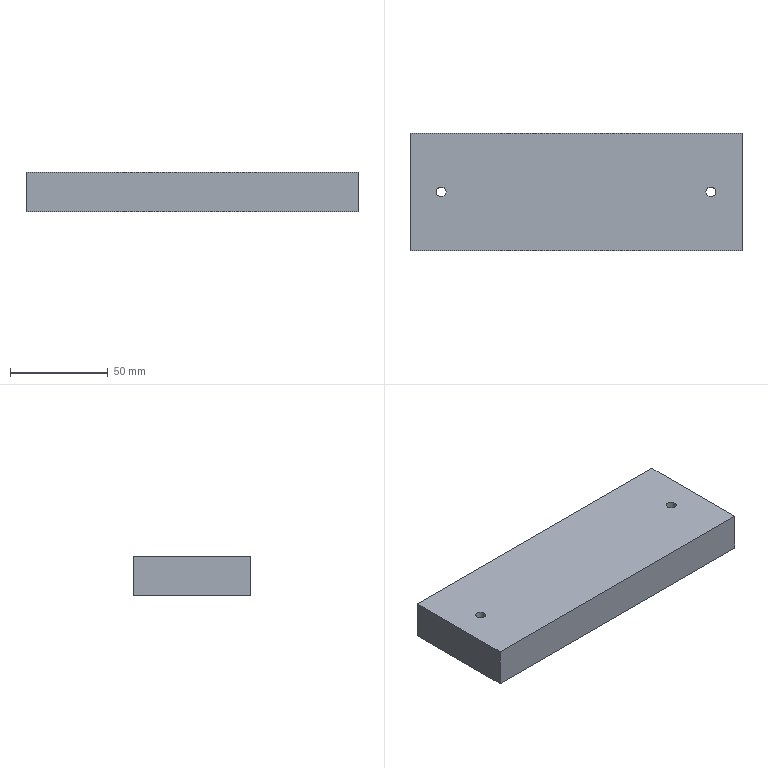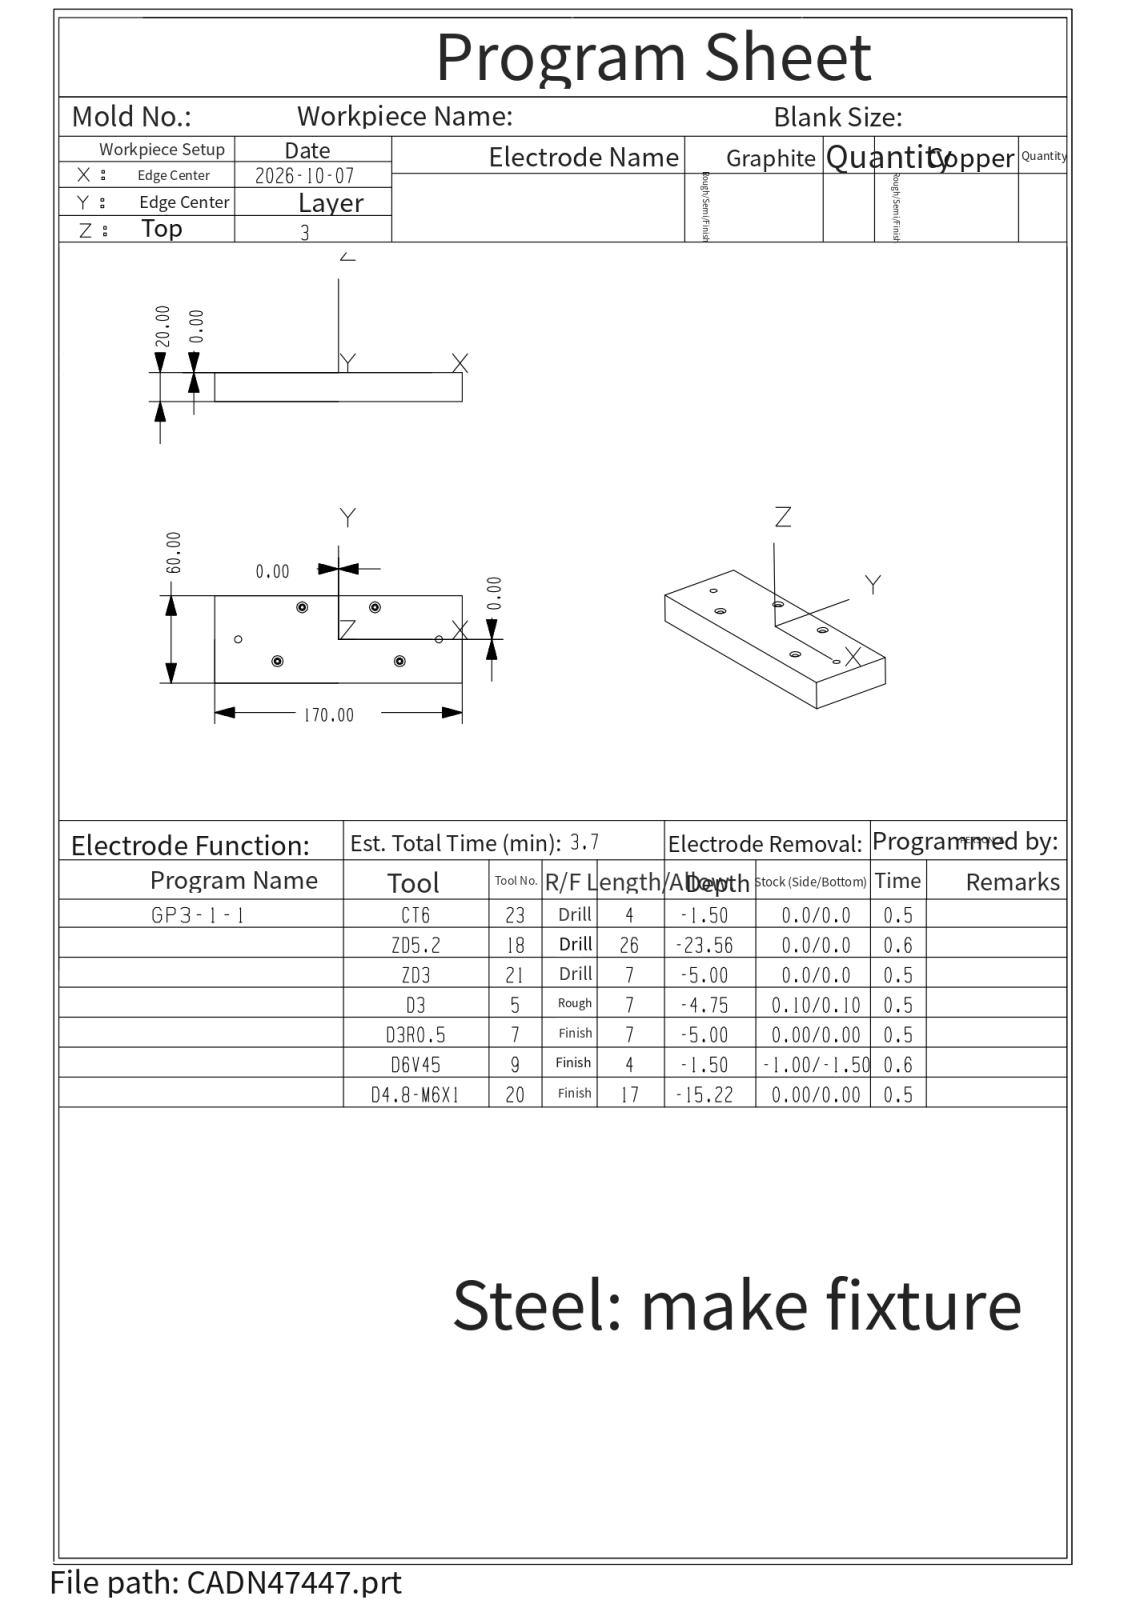NC program | NX | posted by the shop | part box 170 x 60 x 20 mm
Lines 3043 to 4032 of 14163:
T07 M06
T09
( name=D3R0.5    T=7 )
( XY = 0.00 )
( Z = 0.00 )
G00 G90 G54 X-42.899 Y-16.408 S8000 M03
G43 Z10. H07 M08
Z.186
G01 Z-.014 F2400.
Y-16.671
G03 X-41.999 Y-17.571 I.9 J0.0
I0.0 J2.571 F3000.
G01 X-41.917 Y-17.564
X-41.835 Y-17.554 Z-.015
X-41.754 Y-17.542 Z-.016
X-41.673 Y-17.527
X-41.593 Y-17.51 Z-.017
X-41.514 Y-17.49 Z-.018
X-41.436 Y-17.468 Z-.019
X-41.358 Y-17.444
X-41.282 Y-17.417 Z-.02
X-41.206 Y-17.388 Z-.021
X-41.131 Y-17.357
X-41.058 Y-17.323 Z-.022
X-40.986 Y-17.288 Z-.023
X-40.915 Y-17.25 Z-.024
X-40.846 Y-17.21
X-40.778 Y-17.168 Z-.025
X-40.711 Y-17.124 Z-.026
X-40.646 Y-17.077 Z-.027
X-40.583 Y-17.029
X-40.521 Y-16.98 Z-.028
X-40.461 Y-16.928 Z-.029
X-40.402 Y-16.874
X-40.346 Y-16.819 Z-.03
X-40.291 Y-16.762 Z-.031
X-40.239 Y-16.704 Z-.032
X-40.188 Y-16.644
X-40.139 Y-16.582 Z-.033
X-40.092 Y-16.519 Z-.034
X-40.048 Y-16.455
X-40.005 Y-16.389 Z-.035
X-39.965 Y-16.323 Z-.036
X-39.926 Y-16.255 Z-.037
X-39.89 Y-16.186
X-39.857 Y-16.116 Z-.038
G03 X-41.999 Y-17.416 I-2.142 J1.116
G01 X-41.915 Y-17.411 Z-.039
X-41.83 Y-17.402 Z-.04
X-41.747 Y-17.391
X-41.663 Y-17.377 Z-.041
X-41.581 Y-17.361 Z-.042
X-41.499 Y-17.341
X-41.418 Y-17.319 Z-.043
X-41.338 Y-17.294 Z-.044
X-41.259 Y-17.266 Z-.045
X-41.181 Y-17.235
X-41.105 Y-17.202 Z-.046
X-41.029 Y-17.166 Z-.047
X-40.955 Y-17.128 Z-.048
X-40.883 Y-17.087
X-40.812 Y-17.044 Z-.049
X-40.743 Y-16.998 Z-.05
X-40.675 Y-16.95 Z-.051
X-40.61 Y-16.9
X-40.546 Y-16.847 Z-.052
X-40.484 Y-16.793 Z-.053
X-40.424 Y-16.736 Z-.054
X-40.366 Y-16.678
X-40.311 Y-16.617 Z-.055
X-40.257 Y-16.555 Z-.056
X-40.206 Y-16.491 Z-.057
X-40.157 Y-16.425
X-40.111 Y-16.358 Z-.058
X-40.067 Y-16.289 Z-.059
X-40.026 Y-16.219
X-39.987 Y-16.148 Z-.06
X-39.95 Y-16.075 Z-.061
X-39.916 Y-16.001 Z-.062
X-39.885 Y-15.926
X-39.857 Y-15.851 Z-.063
X-39.831 Y-15.774 Z-.064
X-39.808 Y-15.697 Z-.065
X-39.787 Y-15.619
X-39.77 Y-15.54 Z-.066
X-39.755 Y-15.461 Z-.067
X-39.743 Y-15.381 Z-.068
X-39.734 Y-15.302
X-39.727 Y-15.222 Z-.069
X-39.724 Y-15.142 Z-.07
X-39.723 Y-15.062 Z-.071
X-39.725 Y-14.982
X-39.729 Y-14.902 Z-.072
X-39.737 Y-14.823 Z-.073
X-39.747 Y-14.744 Z-.074
G03 X-41.999 Y-17.267 I-2.252 J-.256
G01 X-41.914 Y-17.262
X-41.829 Y-17.255 Z-.075
X-41.744 Y-17.244 Z-.076
X-41.66 Y-17.23 Z-.077
X-41.576 Y-17.213
X-41.493 Y-17.193 Z-.078
X-41.412 Y-17.17 Z-.079
X-41.331 Y-17.144 Z-.08
X-41.251 Y-17.115
X-41.173 Y-17.083 Z-.081
X-41.096 Y-17.048 Z-.082
X-41.02 Y-17.01 Z-.083
X-40.946 Y-16.969
X-40.874 Y-16.926 Z-.084
X-40.803 Y-16.88 Z-.085
X-40.735 Y-16.831
X-40.668 Y-16.78 Z-.086
X-40.603 Y-16.727 Z-.087
X-40.541 Y-16.671 Z-.088
X-40.48 Y-16.613
X-40.422 Y-16.553 Z-.089
X-40.366 Y-16.49 Z-.09
X-40.313 Y-16.426 Z-.091
X-40.262 Y-16.36
X-40.214 Y-16.292 Z-.092
X-40.169 Y-16.222 Z-.093
X-40.126 Y-16.151 Z-.094
X-40.086 Y-16.078
X-40.048 Y-16.004 Z-.095
X-40.014 Y-15.929 Z-.096
X-39.982 Y-15.853 Z-.097
X-39.954 Y-15.775
X-39.928 Y-15.696 Z-.098
X-39.906 Y-15.617 Z-.099
X-39.886 Y-15.537 Z-.1
X-39.869 Y-15.456
X-39.856 Y-15.375 Z-.101
X-39.846 Y-15.294 Z-.102
X-39.838 Y-15.212 Z-.103
X-39.834 Y-15.13
X-39.833 Y-15.048 Z-.104
X-39.835 Y-14.966 Z-.105
X-39.84 Y-14.885 Z-.106
X-39.848 Y-14.803
X-39.859 Y-14.723 Z-.107
X-39.873 Y-14.642 Z-.108
X-39.89 Y-14.563 Z-.109
X-39.91 Y-14.484
X-39.933 Y-14.406 Z-.11
X-39.959 Y-14.329 Z-.111
X-39.988 Y-14.253 Z-.112
X-40.02 Y-14.179
X-40.054 Y-14.106 Z-.113
X-40.091 Y-14.034 Z-.114
X-40.131 Y-13.963 Z-.115
X-40.173 Y-13.895
X-40.218 Y-13.828 Z-.116
X-40.265 Y-13.762 Z-.117
X-40.315 Y-13.699 Z-.118
X-40.367 Y-13.638
X-40.421 Y-13.579 Z-.119
X-40.477 Y-13.521 Z-.12
G03 X-41.999 Y-17.122 I-1.522 J-1.479
G01 X-41.914 Y-17.118 Z-.121
X-41.828 Y-17.111
X-41.743 Y-17.1 Z-.122
X-41.659 Y-17.086 Z-.123
X-41.575 Y-17.069 Z-.124
X-41.492 Y-17.048
X-41.411 Y-17.024 Z-.125
X-41.33 Y-16.996 Z-.126
X-41.251 Y-16.966 Z-.127
X-41.172 Y-16.932
X-41.096 Y-16.895 Z-.128
X-41.021 Y-16.856 Z-.129
X-40.948 Y-16.813 Z-.13
X-40.876 Y-16.767
X-40.807 Y-16.719 Z-.131
X-40.74 Y-16.668 Z-.132
X-40.675 Y-16.614 Z-.133
X-40.612 Y-16.558
X-40.551 Y-16.499 Z-.134
X-40.493 Y-16.438 Z-.135
X-40.438 Y-16.374 Z-.136
X-40.385 Y-16.309
X-40.335 Y-16.241 Z-.137
X-40.288 Y-16.172 Z-.138
X-40.243 Y-16.101 Z-.139
X-40.202 Y-16.028
X-40.164 Y-15.954 Z-.14
X-40.128 Y-15.878 Z-.141
X-40.096 Y-15.801 Z-.142
X-40.067 Y-15.723
X-40.041 Y-15.643 Z-.143
X-40.018 Y-15.563 Z-.144
X-39.999 Y-15.482 Z-.145
X-39.983 Y-15.401
X-39.97 Y-15.319 Z-.146
X-39.961 Y-15.236 Z-.147
X-39.955 Y-15.153 Z-.148
X-39.952 Y-15.071
X-39.953 Y-14.988 Z-.149
X-39.957 Y-14.905 Z-.15
X-39.964 Y-14.823 Z-.151
X-39.975 Y-14.741
X-39.989 Y-14.66 Z-.152
X-40.006 Y-14.579 Z-.153
X-40.026 Y-14.499 Z-.154
X-40.05 Y-14.42
X-40.077 Y-14.343 Z-.155
X-40.106 Y-14.266 Z-.156
X-40.139 Y-14.191 Z-.157
X-40.175 Y-14.117
X-40.214 Y-14.045 Z-.158
X-40.255 Y-13.975 Z-.159
X-40.3 Y-13.906 Z-.16
X-40.347 Y-13.839
X-40.396 Y-13.774 Z-.161
X-40.449 Y-13.712 Z-.162
X-40.503 Y-13.651 Z-.163
X-40.56 Y-13.593
X-40.619 Y-13.537 Z-.164
X-40.681 Y-13.484 Z-.165
X-40.744 Y-13.433 Z-.166
X-40.81 Y-13.385
X-40.877 Y-13.34 Z-.167
X-40.946 Y-13.297 Z-.168
X-41.016 Y-13.258 Z-.169
X-41.088 Y-13.221
X-41.162 Y-13.187 Z-.17
X-41.236 Y-13.156 Z-.171
X-41.312 Y-13.129 Z-.172
X-41.389 Y-13.104
X-41.466 Y-13.082 Z-.173
X-41.545 Y-13.064 Z-.174
X-41.623 Y-13.049 Z-.175
X-41.703 Y-13.037
X-41.783 Y-13.028 Z-.176
X-41.863 Y-13.023 Z-.177
G03 X-41.999 Y-16.982 I-.136 J-1.977
G01 X-41.914 Y-16.978 Z-.178
X-41.829 Y-16.971
X-41.744 Y-16.96 Z-.179
X-41.66 Y-16.946 Z-.18
X-41.577 Y-16.928
X-41.495 Y-16.906 Z-.181
X-41.413 Y-16.881 Z-.182
X-41.333 Y-16.853 Z-.183
X-41.255 Y-16.821
X-41.178 Y-16.786 Z-.184
X-41.102 Y-16.747 Z-.185
X-41.028 Y-16.705 Z-.186
X-40.957 Y-16.661
X-40.887 Y-16.613 Z-.187
X-40.82 Y-16.562 Z-.188
X-40.754 Y-16.509 Z-.189
X-40.691 Y-16.452
X-40.631 Y-16.393 Z-.19
X-40.574 Y-16.332 Z-.191
X-40.519 Y-16.268 Z-.192
X-40.467 Y-16.202
X-40.417 Y-16.134 Z-.193
X-40.371 Y-16.064 Z-.194
X-40.328 Y-15.992 Z-.195
X-40.288 Y-15.919
X-40.252 Y-15.843 Z-.196
X-40.219 Y-15.767 Z-.197
X-40.189 Y-15.688 Z-.198
X-40.162 Y-15.609
X-40.139 Y-15.529 Z-.199
X-40.119 Y-15.448 Z-.2
X-40.103 Y-15.366 Z-.201
X-40.091 Y-15.284
X-40.082 Y-15.201 Z-.202
X-40.077 Y-15.118 Z-.203
X-40.075 Y-15.035 Z-.204
X-40.077 Y-14.952
X-40.082 Y-14.87 Z-.205
X-40.091 Y-14.787 Z-.206
X-40.103 Y-14.705 Z-.207
X-40.119 Y-14.624
X-40.139 Y-14.544 Z-.208
X-40.161 Y-14.465 Z-.209
X-40.188 Y-14.386 Z-.21
X-40.217 Y-14.309
X-40.25 Y-14.234 Z-.211
X-40.286 Y-14.16 Z-.212
X-40.325 Y-14.087 Z-.213
X-40.367 Y-14.017
X-40.412 Y-13.948 Z-.214
X-40.46 Y-13.882 Z-.215
X-40.511 Y-13.817 Z-.216
X-40.565 Y-13.755
X-40.621 Y-13.696 Z-.217
X-40.679 Y-13.638 Z-.218
X-40.74 Y-13.584 Z-.219
X-40.803 Y-13.532
X-40.869 Y-13.483 Z-.22
X-40.936 Y-13.437 Z-.221
X-41.005 Y-13.394 Z-.222
X-41.076 Y-13.354
X-41.148 Y-13.317 Z-.223
X-41.222 Y-13.283 Z-.224
X-41.298 Y-13.252
X-41.374 Y-13.225 Z-.225
X-41.452 Y-13.201 Z-.226
X-41.53 Y-13.181 Z-.227
X-41.609 Y-13.163
X-41.689 Y-13.15 Z-.228
X-41.769 Y-13.139 Z-.229
X-41.85 Y-13.133 Z-.23
X-41.93 Y-13.129
X-42.011 Y-13.13 Z-.231
X-42.092 Y-13.133 Z-.232
X-42.172 Y-13.14 Z-.233
X-42.252 Y-13.151
X-42.331 Y-13.165 Z-.234
X-42.409 Y-13.182 Z-.235
X-42.487 Y-13.203 Z-.236
X-42.564 Y-13.227
X-42.639 Y-13.254 Z-.237
X-42.713 Y-13.285 Z-.238
X-42.786 Y-13.318 Z-.239
X-42.857 Y-13.355
X-42.926 Y-13.395 Z-.24
X-42.994 Y-13.438 Z-.241
X-43.06 Y-13.483 Z-.242
X-43.123 Y-13.531
X-43.185 Y-13.582 Z-.243
X-43.244 Y-13.636 Z-.244
G03 X-41.999 Y-16.847 I1.245 J-1.364
G01 X-41.913 Y-16.843 Z-.245
X-41.828 Y-16.836 Z-.246
X-41.742 Y-16.824
X-41.658 Y-16.809 Z-.247
X-41.574 Y-16.79 Z-.248
X-41.492 Y-16.766 Z-.249
X-41.411 Y-16.739 Z-.25
X-41.331 Y-16.709
X-41.252 Y-16.674 Z-.251
X-41.176 Y-16.636 Z-.252
X-41.101 Y-16.595 Z-.253
X-41.029 Y-16.55 Z-.254
X-40.958 Y-16.502 Z-.255
X-40.89 Y-16.451
X-40.825 Y-16.396 Z-.256
X-40.762 Y-16.339 Z-.257
X-40.702 Y-16.279 Z-.258
X-40.645 Y-16.216 Z-.259
X-40.591 Y-16.151
X-40.54 Y-16.083 Z-.26
X-40.492 Y-16.013 Z-.261
X-40.448 Y-15.941 Z-.262
X-40.407 Y-15.867 Z-.263
X-40.369 Y-15.791 Z-.264
X-40.336 Y-15.714
X-40.306 Y-15.635 Z-.265
X-40.279 Y-15.555 Z-.266
X-40.257 Y-15.474 Z-.267
X-40.238 Y-15.392 Z-.268
X-40.223 Y-15.309
X-40.212 Y-15.226 Z-.269
X-40.205 Y-15.142 Z-.27
X-40.201 Y-15.058 Z-.271
X-40.202 Y-14.974 Z-.272
X-40.207 Y-14.891 Z-.273
X-40.215 Y-14.807
X-40.227 Y-14.725 Z-.274
X-40.243 Y-14.643 Z-.275
X-40.263 Y-14.562 Z-.276
X-40.287 Y-14.482 Z-.277
X-40.314 Y-14.403
X-40.345 Y-14.326 Z-.278
X-40.38 Y-14.25 Z-.279
X-40.418 Y-14.176 Z-.28
X-40.459 Y-14.104 Z-.281
X-40.504 Y-14.034 Z-.282
X-40.551 Y-13.966
X-40.602 Y-13.9 Z-.283
X-40.656 Y-13.837 Z-.284
X-40.713 Y-13.777 Z-.285
X-40.772 Y-13.719 Z-.286
X-40.834 Y-13.664
X-40.898 Y-13.613 Z-.287
X-40.965 Y-13.564 Z-.288
X-41.034 Y-13.518 Z-.289
X-41.104 Y-13.476 Z-.29
X-41.177 Y-13.437 Z-.291
X-41.251 Y-13.402
X-41.327 Y-13.37 Z-.292
X-41.404 Y-13.342 Z-.293
X-41.483 Y-13.317 Z-.294
X-41.562 Y-13.296 Z-.295
X-41.642 Y-13.279
X-41.723 Y-13.266 Z-.296
X-41.804 Y-13.256 Z-.297
X-41.886 Y-13.25 Z-.298
X-41.967 Y-13.248 Z-.299
X-42.049 Y-13.25 Z-.3
X-42.13 Y-13.255
X-42.211 Y-13.265 Z-.301
X-42.292 Y-13.278 Z-.302
X-42.372 Y-13.294 Z-.303
X-42.45 Y-13.315 Z-.304
X-42.528 Y-13.339
X-42.604 Y-13.367 Z-.305
X-42.679 Y-13.398 Z-.306
X-42.753 Y-13.432 Z-.307
X-42.824 Y-13.47 Z-.308
X-42.894 Y-13.512 Z-.309
X-42.962 Y-13.556
X-43.027 Y-13.603 Z-.31
X-43.09 Y-13.654 Z-.311
X-43.151 Y-13.707 Z-.312
X-43.209 Y-13.763 Z-.313
X-43.264 Y-13.822 Z-.314
X-43.317 Y-13.883
X-43.367 Y-13.946 Z-.315
X-43.413 Y-14.012 Z-.316
X-43.457 Y-14.079 Z-.317
X-43.497 Y-14.149 Z-.318
X-43.534 Y-14.22
X-43.567 Y-14.293 Z-.319
X-43.597 Y-14.368 Z-.32
X-43.624 Y-14.443 Z-.321
G03 X-41.999 Y-16.717 I1.625 J-.557
G01 X-41.914 Y-16.714 Z-.322
X-41.829 Y-16.706 Z-.323
X-41.745 Y-16.694 Z-.324
X-41.661 Y-16.678 Z-.325
X-41.579 Y-16.657 Z-.326
X-41.497 Y-16.633 Z-.327
X-41.417 Y-16.605 Z-.328
X-41.339 Y-16.572 Z-.329
X-41.262 Y-16.536 Z-.33
X-41.187 Y-16.496 Z-.331
X-41.115 Y-16.453 Z-.332
X-41.045 Y-16.406 Z-.333
X-40.977 Y-16.356 Z-.334
X-40.912 Y-16.302 Z-.335
X-40.849 Y-16.245 Z-.336
X-40.79 Y-16.185 Z-.337
X-40.734 Y-16.123 Z-.338
X-40.68 Y-16.058 Z-.339
X-40.631 Y-15.99 Z-.34
X-40.584 Y-15.92 Z-.341
X-40.542 Y-15.848
X-40.503 Y-15.774 Z-.342
X-40.467 Y-15.698 Z-.343
X-40.436 Y-15.62 Z-.344
X-40.408 Y-15.541 Z-.345
X-40.385 Y-15.461 Z-.346
X-40.365 Y-15.38 Z-.347
X-40.35 Y-15.298 Z-.348
X-40.339 Y-15.216 Z-.349
X-40.331 Y-15.133 Z-.35
X-40.328 Y-15.05 Z-.351
X-40.329 Y-14.967 Z-.352
X-40.334 Y-14.884 Z-.353
X-40.344 Y-14.801 Z-.354
X-40.357 Y-14.72 Z-.355
X-40.374 Y-14.639 Z-.356
X-40.396 Y-14.559 Z-.357
X-40.421 Y-14.48 Z-.358
X-40.45 Y-14.403 Z-.359
X-40.483 Y-14.327 Z-.36
X-40.519 Y-14.253 Z-.361
X-40.559 Y-14.181 Z-.362
X-40.603 Y-14.112 Z-.363
X-40.65 Y-14.044 Z-.364
X-40.7 Y-13.979 Z-.365
X-40.754 Y-13.917 Z-.366
X-40.81 Y-13.857 Z-.367
X-40.869 Y-13.8 Z-.368
X-40.931 Y-13.747 Z-.369
X-40.996 Y-13.696 Z-.37
X-41.062 Y-13.649 Z-.371
X-41.131 Y-13.606 Z-.372
X-41.202 Y-13.565 Z-.373
X-41.275 Y-13.529 Z-.374
X-41.35 Y-13.496 Z-.375
X-41.426 Y-13.467 Z-.376
X-41.503 Y-13.442 Z-.377
X-41.582 Y-13.42 Z-.378
X-41.661 Y-13.403 Z-.379
X-41.741 Y-13.389 Z-.38
X-41.821 Y-13.38 Z-.381
X-41.902 Y-13.374 Z-.382
X-41.983 Y-13.373 Z-.383
X-42.064 Y-13.375 Z-.384
X-42.144 Y-13.382 Z-.385
X-42.225 Y-13.392 Z-.386
X-42.304 Y-13.407 Z-.387
X-42.382 Y-13.425 Z-.388
X-42.46 Y-13.448 Z-.389
X-42.536 Y-13.474 Z-.39
X-42.611 Y-13.503 Z-.391
X-42.684 Y-13.537 Z-.392
X-42.755 Y-13.574 Z-.393
X-42.824 Y-13.614 Z-.394
X-42.891 Y-13.658 Z-.395
X-42.956 Y-13.705 Z-.396
X-43.018 Y-13.755
X-43.078 Y-13.809 Z-.397
X-43.135 Y-13.864 Z-.398
X-43.189 Y-13.923 Z-.399
X-43.24 Y-13.984 Z-.4
X-43.288 Y-14.048 Z-.401
X-43.332 Y-14.114 Z-.402
X-43.374 Y-14.182 Z-.403
X-43.412 Y-14.252 Z-.404
X-43.446 Y-14.324 Z-.405
X-43.476 Y-14.397 Z-.406
X-43.503 Y-14.472 Z-.407
G03 X-41.999 Y-16.594 I1.504 J-.528
G01 X-41.914 Y-16.59 Z-.408
X-41.83 Y-16.582 Z-.41
X-41.746 Y-16.569 Z-.411
X-41.663 Y-16.552 Z-.412
X-41.582 Y-16.531 Z-.413
X-41.501 Y-16.505 Z-.414
X-41.422 Y-16.475 Z-.415
X-41.345 Y-16.441 Z-.417
X-41.27 Y-16.402 Z-.418
X-41.197 Y-16.36 Z-.419
X-41.127 Y-16.314 Z-.42
X-41.059 Y-16.265 Z-.421
X-40.994 Y-16.212 Z-.422
X-40.932 Y-16.155 Z-.424
X-40.873 Y-16.096 Z-.425
X-40.817 Y-16.033 Z-.426
X-40.765 Y-15.968 Z-.427
X-40.716 Y-15.9 Z-.428
X-40.671 Y-15.83 Z-.429
X-40.63 Y-15.757 Z-.431
X-40.593 Y-15.683 Z-.432
X-40.56 Y-15.606 Z-.433
X-40.531 Y-15.528 Z-.434
X-40.507 Y-15.449 Z-.435
X-40.486 Y-15.368 Z-.436
X-40.47 Y-15.287 Z-.438
X-40.459 Y-15.205 Z-.439
X-40.451 Y-15.122 Z-.44
X-40.449 Y-15.04 Z-.441
X-40.45 Y-14.957 Z-.442
X-40.456 Y-14.875 Z-.443
X-40.466 Y-14.793 Z-.444
X-40.481 Y-14.712 Z-.446
X-40.5 Y-14.632 Z-.447
X-40.523 Y-14.553 Z-.448
X-40.55 Y-14.476 Z-.449
X-40.581 Y-14.4 Z-.45
X-40.617 Y-14.326 Z-.451
X-40.656 Y-14.254 Z-.453
X-40.699 Y-14.184 Z-.454
X-40.745 Y-14.117 Z-.455
X-40.795 Y-14.052 Z-.456
X-40.848 Y-13.99 Z-.457
X-40.905 Y-13.931 Z-.458
X-40.964 Y-13.876 Z-.46
X-41.026 Y-13.823 Z-.461
X-41.091 Y-13.774 Z-.462
X-41.159 Y-13.729 Z-.463
X-41.228 Y-13.687 Z-.464
X-41.3 Y-13.649 Z-.465
X-41.373 Y-13.615 Z-.467
X-41.449 Y-13.585 Z-.468
X-41.525 Y-13.559 Z-.469
X-41.603 Y-13.537 Z-.47
X-41.682 Y-13.519 Z-.471
X-41.761 Y-13.506 Z-.472
X-41.841 Y-13.497 Z-.474
X-41.922 Y-13.492 Z-.475
X-42.002 Y-13.491 Z-.476
X-42.082 Y-13.495 Z-.477
X-42.162 Y-13.503 Z-.478
X-42.241 Y-13.515 Z-.479
X-42.32 Y-13.531 Z-.481
X-42.397 Y-13.552 Z-.482
X-42.473 Y-13.576 Z-.483
X-42.548 Y-13.605 Z-.484
X-42.621 Y-13.637 Z-.485
X-42.692 Y-13.673 Z-.486
X-42.761 Y-13.713 Z-.488
X-42.828 Y-13.757 Z-.489
X-42.892 Y-13.804 Z-.49
X-42.954 Y-13.854 Z-.491
X-43.012 Y-13.908 Z-.492
X-43.068 Y-13.964 Z-.493
X-43.121 Y-14.023 Z-.495
X-43.17 Y-14.085 Z-.496
X-43.216 Y-14.15 Z-.497
X-43.259 Y-14.216 Z-.498
X-43.297 Y-14.285 Z-.499
X-43.332 Y-14.356 Z-.5
X-43.364 Y-14.428 Z-.501
X-43.391 Y-14.502 Z-.503
G03 X-41.999 Y-16.478 I1.392 J-.498
G01 X-41.915 Y-16.474 Z-.504
X-41.83 Y-16.465 Z-.505
X-41.747 Y-16.452 Z-.507
X-41.664 Y-16.433 Z-.508
X-41.583 Y-16.41 Z-.509
X-41.503 Y-16.382 Z-.511
X-41.425 Y-16.35 Z-.512
X-41.349 Y-16.314 Z-.514
X-41.275 Y-16.273 Z-.515
X-41.204 Y-16.228 Z-.516
X-41.136 Y-16.179 Z-.518
X-41.071 Y-16.126 Z-.519
X-41.009 Y-16.07 Z-.52
X-40.95 Y-16.011 Z-.522
X-40.895 Y-15.948 Z-.523
X-40.843 Y-15.882 Z-.524
X-40.796 Y-15.813 Z-.526
X-40.752 Y-15.742 Z-.527
X-40.713 Y-15.668 Z-.529
X-40.678 Y-15.593 Z-.53
X-40.648 Y-15.516 Z-.531
X-40.622 Y-15.437 Z-.533
X-40.6 Y-15.357 Z-.534
X-40.584 Y-15.275 Z-.535
X-40.572 Y-15.193 Z-.537
X-40.564 Y-15.111 Z-.538
X-40.562 Y-15.028 Z-.54
X-40.564 Y-14.946 Z-.541
X-40.571 Y-14.864 Z-.542
X-40.583 Y-14.782 Z-.544
X-40.599 Y-14.702 Z-.545
X-40.62 Y-14.622 Z-.546
X-40.645 Y-14.544 Z-.548
X-40.675 Y-14.467 Z-.549
X-40.709 Y-14.393 Z-.55
X-40.747 Y-14.32 Z-.552
X-40.789 Y-14.251 Z-.553
X-40.836 Y-14.183 Z-.555
X-40.886 Y-14.119 Z-.556
X-40.939 Y-14.057 Z-.557
X-40.996 Y-13.999 Z-.559
X-41.056 Y-13.944 Z-.56
X-41.119 Y-13.892 Z-.561
X-41.185 Y-13.845 Z-.563
X-41.253 Y-13.801 Z-.564
X-41.324 Y-13.762 Z-.565
X-41.397 Y-13.726 Z-.567
X-41.472 Y-13.695 Z-.568
X-41.548 Y-13.668 Z-.57
X-41.625 Y-13.646 Z-.571
X-41.704 Y-13.628 Z-.572
X-41.784 Y-13.615 Z-.574
X-41.864 Y-13.606 Z-.575
X-41.944 Y-13.602 Z-.576
X-42.024 Z-.578
X-42.104 Y-13.608 Z-.579
X-42.184 Y-13.617 Z-.58
X-42.263 Y-13.631 Z-.582
X-42.341 Y-13.65 Z-.583
X-42.417 Y-13.673 Z-.585
X-42.492 Y-13.701 Z-.586
X-42.565 Y-13.732 Z-.587
X-42.637 Y-13.768 Z-.589
X-42.706 Y-13.808 Z-.59
X-42.772 Y-13.852 Z-.591
X-42.836 Y-13.899 Z-.593
X-42.897 Y-13.95 Z-.594
X-42.955 Y-14.004 Z-.595
X-43.009 Y-14.062 Z-.597
X-43.061 Y-14.122 Z-.598
X-43.108 Y-14.185 Z-.6
X-43.152 Y-14.251 Z-.601
X-43.192 Y-14.319 Z-.602
X-43.228 Y-14.389 Z-.604
X-43.26 Y-14.461 Z-.605
X-43.287 Y-14.535 Z-.606
G03 X-41.999 Y-16.369 I1.288 J-.465
G01 X-41.914 Y-16.365 Z-.608
X-41.829 Y-16.356 Z-.61
X-41.745 Y-16.341 Z-.611
X-41.663 Y-16.321 Z-.613
X-41.581 Y-16.296 Z-.614
X-41.502 Y-16.266 Z-.616
X-41.425 Y-16.231 Z-.618
X-41.35 Y-16.192 Z-.619
X-41.278 Y-16.148 Z-.621
X-41.208 Y-16.099 Z-.622
X-41.142 Y-16.047 Z-.624
X-41.08 Y-15.99 Z-.626
X-41.021 Y-15.93 Z-.627
X-40.966 Y-15.866 Z-.629
X-40.915 Y-15.799 Z-.63
X-40.869 Y-15.729 Z-.632
X-40.827 Y-15.656 Z-.634
X-40.79 Y-15.581 Z-.635
X-40.757 Y-15.504 Z-.637
X-40.729 Y-15.425 Z-.638
X-40.707 Y-15.345 Z-.64
X-40.689 Y-15.263 Z-.641
X-40.677 Y-15.181 Z-.643
X-40.67 Y-15.098 Z-.645
X-40.668 Y-15.015 Z-.646
X-40.671 Y-14.932 Z-.648
X-40.679 Y-14.85 Z-.649
X-40.692 Y-14.768 Z-.651
X-40.711 Y-14.687 Z-.653
X-40.734 Y-14.608 Z-.654
X-40.762 Y-14.53 Z-.656
X-40.795 Y-14.455 Z-.657
X-40.833 Y-14.382 Z-.659
X-40.875 Y-14.311 Z-.661
X-40.921 Y-14.243 Z-.662
X-40.972 Y-14.178 Z-.664
X-41.026 Y-14.117 Z-.665
X-41.084 Y-14.059 Z-.667
X-41.145 Y-14.004 Z-.669
X-41.21 Y-13.954 Z-.67
X-41.277 Y-13.908 Z-.672
X-41.348 Y-13.867 Z-.673
X-41.42 Y-13.83 Z-.675
X-41.495 Y-13.797 Z-.677
X-41.571 Y-13.769 Z-.678
X-41.649 Y-13.746 Z-.68
X-41.728 Y-13.728 Z-.681
X-41.808 Y-13.715 Z-.683
X-41.889 Y-13.707 Z-.685
X-41.97 Y-13.704 Z-.686
X-42.05 Y-13.706 Z-.688
X-42.131 Y-13.713 Z-.689
X-42.211 Y-13.726 Z-.691
X-42.289 Y-13.743 Z-.692
X-42.367 Y-13.764 Z-.694
X-42.443 Y-13.791 Z-.696
X-42.517 Y-13.822 Z-.697
X-42.588 Y-13.858 Z-.699
X-42.658 Y-13.898 Z-.7
X-42.724 Y-13.942 Z-.702
X-42.788 Y-13.991 Z-.704
X-42.849 Y-14.043 Z-.705
X-42.906 Y-14.099 Z-.707
X-42.959 Y-14.158 Z-.708
X-43.008 Y-14.22 Z-.71
X-43.054 Y-14.285 Z-.712
X-43.095 Y-14.353 Z-.713
X-43.132 Y-14.423 Z-.715
X-43.165 Y-14.496 Z-.716
X-43.193 Y-14.57 Z-.718
G03 X-41.999 Y-16.269 I1.194 J-.43
G01 X-41.915 Y-16.265 Z-.72
X-41.832 Y-16.255 Z-.722
X-41.75 Y-16.24 Z-.723
X-41.669 Y-16.219 Z-.725
X-41.589 Y-16.193 Z-.727
X-41.512 Y-16.162 Z-.729
X-41.437 Y-16.126 Z-.731
X-41.364 Y-16.085 Z-.732
X-41.294 Y-16.039 Z-.734
X-41.228 Y-15.989 Z-.736
X-41.165 Y-15.935 Z-.738
X-41.106 Y-15.876 Z-.74
X-41.051 Y-15.814 Z-.741
X-41.001 Y-15.749 Z-.743
X-40.955 Y-15.681 Z-.745
X-40.913 Y-15.609 Z-.747
X-40.876 Y-15.535 Z-.749
X-40.845 Y-15.459 Z-.75
X-40.818 Y-15.381 Z-.752
X-40.797 Y-15.302 Z-.754
X-40.781 Y-15.222 Z-.756
X-40.771 Y-15.14 Z-.758
X-40.765 Y-15.059 Z-.759
X-40.766 Y-14.977 Z-.761
X-40.771 Y-14.895 Z-.763
X-40.782 Y-14.815 Z-.765
X-40.799 Y-14.735 Z-.767
X-40.82 Y-14.656 Z-.768
X-40.847 Y-14.58 Z-.77
X-40.878 Y-14.505 Z-.772
X-40.915 Y-14.432 Z-.774
X-40.956 Y-14.362 Z-.776
X-41.002 Y-14.296 Z-.777
X-41.052 Y-14.232 Z-.779
X-41.105 Y-14.172 Z-.781
X-41.163 Y-14.116 Z-.783
X-41.224 Y-14.063 Z-.785
X-41.289 Y-14.015 Z-.786
X-41.356 Y-13.972 Z-.788
X-41.427 Y-13.932 Z-.79
X-41.499 Y-13.898 Z-.792
X-41.574 Y-13.869 Z-.794
X-41.65 Y-13.844 Z-.795
X-41.727 Y-13.825 Z-.797
X-41.806 Y-13.811 Z-.799
X-41.885 Y-13.802 Z-.801
X-41.965 Y-13.798 Z-.803
X-42.044 Y-13.8 Z-.804
X-42.123 Y-13.807 Z-.806
X-42.202 Y-13.819 Z-.808
X-42.279 Y-13.837 Z-.81
X-42.355 Y-13.859 Z-.812
X-42.429 Y-13.886 Z-.813
X-42.502 Y-13.918 Z-.815
X-42.571 Y-13.955 Z-.817
X-42.639 Y-13.996 Z-.819
X-42.703 Y-14.042 Z-.821
X-42.764 Y-14.092 Z-.822
X-42.821 Y-14.145 Z-.824
X-42.875 Y-14.202 Z-.826
X-42.925 Y-14.263 Z-.828
X-42.971 Y-14.327 Z-.83
X-43.012 Y-14.393 Z-.831
X-43.049 Y-14.462 Z-.833
X-43.081 Y-14.533 Z-.835
X-43.108 Y-14.606 Z-.837
G03 X-41.999 Y-16.177 I1.109 J-.394
G01 X-41.914 Y-16.172 Z-.839
X-41.828 Y-16.162 Z-.841
X-41.744 Y-16.145 Z-.843
X-41.662 Y-16.121 Z-.845
X-41.582 Y-16.093 Z-.847
X-41.504 Y-16.058 Z-.849
X-41.429 Y-16.018 Z-.851
X-41.357 Y-15.972 Z-.853
X-41.288 Y-15.921 Z-.856
X-41.224 Y-15.866 Z-.858
X-41.164 Y-15.806 Z-.86
X-41.108 Y-15.742 Z-.862
X-41.058 Y-15.674 Z-.864
X-41.012 Y-15.603 Z-.866
X-40.972 Y-15.529 Z-.868
X-40.938 Y-15.452 Z-.87
X-40.909 Y-15.373 Z-.872
X-40.886 Y-15.292 Z-.874
X-40.869 Y-15.21 Z-.876
X-40.858 Y-15.126 Z-.879
X-40.853 Y-15.043 Z-.881
X-40.855 Y-14.959 Z-.883
X-40.862 Y-14.876 Z-.885
X-40.876 Y-14.793 Z-.887
X-40.895 Y-14.713 Z-.889
X-40.92 Y-14.633 Z-.891
X-40.951 Y-14.556 Z-.893
X-40.988 Y-14.481 Z-.895
X-41.029 Y-14.41 Z-.897
X-41.076 Y-14.341 Z-.899
X-41.128 Y-14.277 Z-.901
X-41.184 Y-14.216 Z-.904
X-41.244 Y-14.159 Z-.906
X-41.308 Y-14.108 Z-.908
X-41.376 Y-14.061 Z-.91
X-41.447 Y-14.019 Z-.912
X-41.52 Y-13.983 Z-.914
X-41.597 Y-13.952 Z-.916
X-41.674 Y-13.926 Z-.918
X-41.754 Y-13.907 Z-.92
X-41.834 Y-13.893 Z-.922
X-41.916 Y-13.885 Z-.924
X-41.997 Y-13.884 Z-.927
X-42.079 Y-13.888 Z-.929
X-42.159 Y-13.898 Z-.931
X-42.239 Y-13.914 Z-.933
X-42.317 Y-13.935 Z-.935
X-42.394 Y-13.963 Z-.937
X-42.468 Y-13.995 Z-.939
X-42.539 Y-14.033 Z-.941
X-42.608 Y-14.076 Z-.943
X-42.673 Y-14.124 Z-.945
X-42.734 Y-14.177 Z-.947
X-42.791 Y-14.234 Z-.95
X-42.844 Y-14.294 Z-.952
X-42.892 Y-14.358 Z-.954
X-42.935 Y-14.426 Z-.956
X-42.974 Y-14.496 Z-.958
X-43.007 Y-14.569 Z-.96
X-43.034 Y-14.644 Z-.962
G03 X-41.999 Y-16.094 I1.035 J-.356
G01 X-41.914 Y-16.09 Z-.964
X-41.828 Y-16.078 Z-.967
X-41.745 Y-16.06 Z-.969
X-41.663 Y-16.035 Z-.971
X-41.583 Y-16.005 Z-.974
X-41.506 Y-15.968 Z-.976
X-41.433 Y-15.925 Z-.978
X-41.363 Y-15.876 Z-.981
X-41.297 Y-15.823 Z-.983
X-41.235 Y-15.764 Z-.985
X-41.179 Y-15.701 Z-.988
X-41.127 Y-15.633 Z-.99
X-41.082 Y-15.562 Z-.992
X-41.042 Y-15.488 Z-.995
X-41.007 Y-15.411 Z-.997
X-40.98 Y-15.331 Z-1.
X-40.958 Y-15.25 Z-1.002
X-40.943 Y-15.167 Z-1.004
X-40.934 Y-15.084 Z-1.007
X-40.932 Y-15. Z-1.009
X-40.937 Y-14.917 Z-1.011
X-40.948 Y-14.834 Z-1.014
X-40.966 Y-14.752 Z-1.016
X-40.99 Y-14.672 Z-1.018
X-41.02 Y-14.595 Z-1.021
X-41.056 Y-14.519 Z-1.023
X-41.097 Y-14.448 Z-1.025
X-41.145 Y-14.379 Z-1.028
X-41.197 Y-14.315 Z-1.03
X-41.254 Y-14.255 Z-1.032
X-41.316 Y-14.2 Z-1.035
X-41.381 Y-14.15 Z-1.037
X-41.45 Y-14.105 Z-1.039
X-41.523 Y-14.066 Z-1.042
X-41.598 Y-14.033 Z-1.044
X-41.676 Y-14.005 Z-1.046
X-41.755 Y-13.984 Z-1.049
X-41.836 Y-13.969 Z-1.051
X-41.917 Y-13.961 Z-1.053
X-41.999 Y-13.959 Z-1.056
X-42.08 Y-13.964 Z-1.058
X-42.161 Y-13.974 Z-1.06
X-42.241 Y-13.991 Z-1.063
X-42.319 Y-14.015 Z-1.065
X-42.395 Y-14.044 Z-1.067
X-42.468 Y-14.079 Z-1.07
X-42.538 Y-14.12 Z-1.072
X-42.605 Y-14.166 Z-1.074
X-42.668 Y-14.217 Z-1.077
X-42.726 Y-14.273 Z-1.079
X-42.78 Y-14.333 Z-1.081
X-42.829 Y-14.397 Z-1.084
X-42.873 Y-14.464 Z-1.086
X-42.911 Y-14.535 Z-1.088
X-42.944 Y-14.608 Z-1.091
X-42.97 Y-14.684 Z-1.093
G03 X-41.999 Y-16.021 I.971 J-.316
G01 X-41.916 Y-16.017 Z-1.096
X-41.833 Y-16.005 Z-1.098
X-41.752 Y-15.987 Z-1.101
X-41.672 Y-15.962 Z-1.103
X-41.595 Y-15.931 Z-1.106
X-41.521 Y-15.894 Z-1.108
X-41.45 Y-15.851 Z-1.111
X-41.383 Y-15.802 Z-1.113
X-41.321 Y-15.748 Z-1.116
X-41.262 Y-15.689 Z-1.118
X-41.21 Y-15.626 Z-1.121
X-41.162 Y-15.558 Z-1.123
X-41.12 Y-15.487 Z-1.126
X-41.084 Y-15.413 Z-1.128
X-41.055 Y-15.337 Z-1.131
X-41.032 Y-15.258 Z-1.134
X-41.015 Y-15.178 Z-1.136
X-41.005 Y-15.097 Z-1.139
X-41.002 Y-15.015 Z-1.141
X-41.005 Y-14.933 Z-1.144
X-41.015 Y-14.853 Z-1.146
X-41.031 Y-14.773 Z-1.149
X-41.054 Y-14.695 Z-1.151
X-41.084 Y-14.619 Z-1.154
X-41.119 Y-14.546 Z-1.156
X-41.16 Y-14.476 Z-1.159
X-41.206 Y-14.41 Z-1.161
X-41.258 Y-14.348 Z-1.164
X-41.315 Y-14.29 Z-1.166
X-41.376 Y-14.237 Z-1.169
X-41.441 Y-14.19 Z-1.171
X-41.51 Y-14.148 Z-1.174
X-41.582 Y-14.112 Z-1.176
X-41.656 Y-14.082 Z-1.179
X-41.733 Y-14.058 Z-1.181
X-41.811 Y-14.04 Z-1.184
X-41.89 Y-14.029 Z-1.187
X-41.97 Y-14.025 Z-1.189
X-42.05 Y-14.027 Z-1.192
X-42.129 Y-14.035 Z-1.194
X-42.207 Y-14.05 Z-1.197
X-42.284 Y-14.071 Z-1.199
X-42.359 Y-14.099 Z-1.202
X-42.431 Y-14.132 Z-1.204
X-42.5 Y-14.171 Z-1.207
X-42.565 Y-14.216 Z-1.209
X-42.627 Y-14.266 Z-1.212
X-42.684 Y-14.32 Z-1.214
X-42.736 Y-14.379 Z-1.217
X-42.784 Y-14.442 Z-1.219
X-42.826 Y-14.509 Z-1.222
X-42.862 Y-14.578 Z-1.224
X-42.893 Y-14.651 Z-1.227
X-42.917 Y-14.725 Z-1.229
G03 X-41.999 Y-15.958 I.918 J-.275
G01 X-41.914 Y-15.953 Z-1.232
X-41.83 Y-15.941 Z-1.235
X-41.747 Y-15.921 Z-1.238
X-41.667 Y-15.894 Z-1.241
X-41.589 Y-15.86 Z-1.243
X-41.515 Y-15.819 Z-1.246
X-41.444 Y-15.771 Z-1.249
X-41.379 Y-15.718 Z-1.252